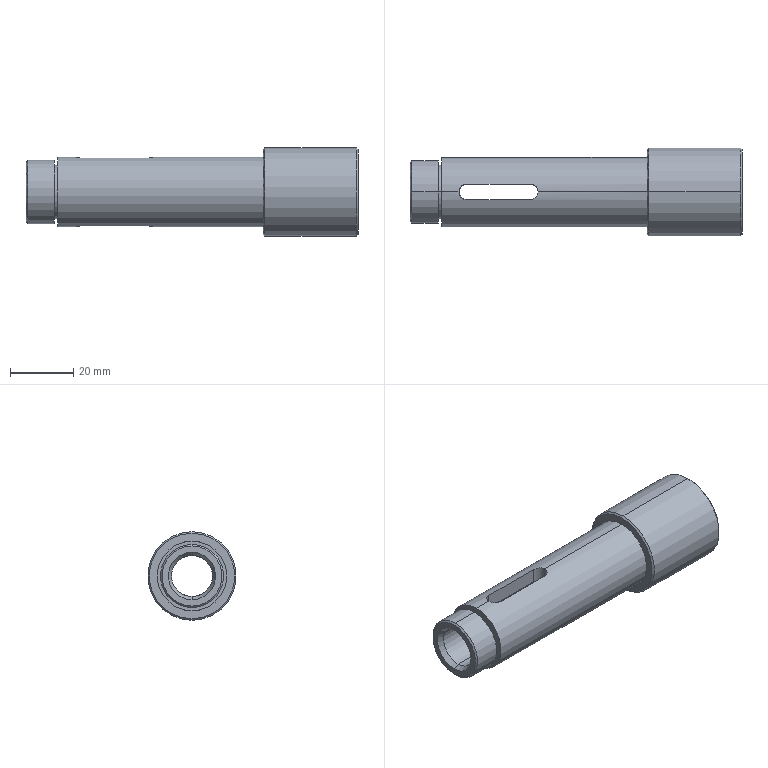Part | SolidWorks | features ICE 3, Chamfer 2, Extrusion 1, HoleWzd 1, RevCut 1 | 1 solid | 43 faces | box 105 x 28 x 28 mm | volume 30891 mm3 | cylinder 20 | cone 14 | plane 9 | commonest cylinder face diameters 5 x6 4 x4 13 x2 17 x2 20 x2 22 x2